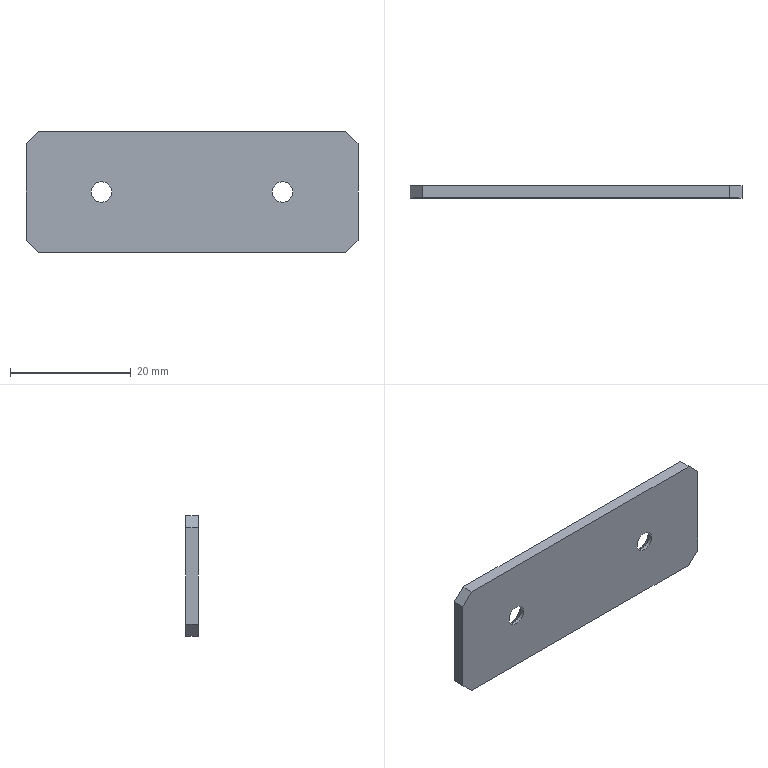Part | STEP file | Part1.SLDPRTrtt_Default | 1 solid | 18 faces | box 55 x 2 x 20 mm | volume 2119 mm3 | plane 10 | cone 4 | cylinder 4 | commonest cylinder face diameters 3.4 x4
STEP:
#1=CARTESIAN_POINT('',(0.,0.,0.));
#2=DIRECTION('',(0.,0.,1.));
#3=DIRECTION('',(1.,0.,0.));
#4=AXIS2_PLACEMENT_3D('',#1,#2,#3);
#5=CARTESIAN_POINT('',(-15.,0.55,1.7));
#6=VERTEX_POINT('',#5);
#7=CARTESIAN_POINT('',(-15.,2.,3.15));
#8=VERTEX_POINT('',#7);
#9=CARTESIAN_POINT('',(-15.,2.,3.15));
#10=DIRECTION('',(0.,0.7071,0.7071));
#11=VECTOR('',#10,1.);
#12=LINE('',#9,#11);
#13=CARTESIAN_POINT('',(-15.,2.,0.));
#14=DIRECTION('',(0.,1.,0.));
#15=DIRECTION('',(0.,0.,1.));
#16=AXIS2_PLACEMENT_3D('',#13,#14,#15);
#17=CONICAL_SURFACE('',#16,3.15,0.7854);
#18=CARTESIAN_POINT('',(6.283,0.));
#19=DIRECTION('',(0.,1.));
#20=VECTOR('',#19,1.);
#21=LINE('',#18,#20);
#22=(GEOMETRIC_REPRESENTATION_CONTEXT(2)PARAMETRIC_REPRESENTATION_CONTEXT()REPRESENTATION_CONTEXT('',''));
#23=DEFINITIONAL_REPRESENTATION('',(#21),#22);
#24=PCURVE('',#17,#23);
#25=CARTESIAN_POINT('',(-15.,2.,0.));
#26=DIRECTION('',(0.,1.,0.));
#27=DIRECTION('',(0.,0.,1.));
#28=AXIS2_PLACEMENT_3D('',#25,#26,#27);
#29=CONICAL_SURFACE('',#28,3.15,0.7854);
#30=CARTESIAN_POINT('',(0.,0.));
#31=DIRECTION('',(0.,1.));
#32=VECTOR('',#31,1.);
#33=LINE('',#30,#32);
#34=(GEOMETRIC_REPRESENTATION_CONTEXT(2)PARAMETRIC_REPRESENTATION_CONTEXT()REPRESENTATION_CONTEXT('',''));
#35=DEFINITIONAL_REPRESENTATION('',(#33),#34);
#36=PCURVE('',#29,#35);
#37=SURFACE_CURVE('',#12,(#24,#36),.PCURVE_S1.);
#38=EDGE_CURVE('',#6,#8,#37,.T.);
#39=ORIENTED_EDGE('',*,*,#38,.T.);
#40=CARTESIAN_POINT('',(-15.,2.,-3.15));
#41=VERTEX_POINT('',#40);
#42=CARTESIAN_POINT('',(-15.,2.,0.));
#43=DIRECTION('',(0.,1.,0.));
#44=DIRECTION('',(0.,0.,1.));
#45=AXIS2_PLACEMENT_3D('',#42,#43,#44);
#46=CIRCLE('',#45,3.15);
#47=CARTESIAN_POINT('',(0.,0.));
#48=DIRECTION('',(1.,0.));
#49=VECTOR('',#48,1.);
#50=LINE('',#47,#49);
#51=(GEOMETRIC_REPRESENTATION_CONTEXT(2)PARAMETRIC_REPRESENTATION_CONTEXT()REPRESENTATION_CONTEXT('',''));
#52=DEFINITIONAL_REPRESENTATION('',(#50),#51);
#53=PCURVE('',#17,#52);
#54=CARTESIAN_POINT('',(0.,2.,0.));
#55=DIRECTION('',(0.,1.,0.));
#56=DIRECTION('',(0.,0.,1.));
#57=AXIS2_PLACEMENT_3D('',#54,#55,#56);
#58=PLANE('',#57);
#59=CARTESIAN_POINT('',(0.,-15.));
#60=DIRECTION('',(1.,0.));
#61=AXIS2_PLACEMENT_2D('',#59,#60);
#62=CIRCLE('',#61,3.15);
#63=(GEOMETRIC_REPRESENTATION_CONTEXT(2)PARAMETRIC_REPRESENTATION_CONTEXT()REPRESENTATION_CONTEXT('',''));
#64=DEFINITIONAL_REPRESENTATION('',(#62),#63);
#65=PCURVE('',#58,#64);
#66=SURFACE_CURVE('',#46,(#53,#65),.PCURVE_S1.);
#67=EDGE_CURVE('',#41,#8,#66,.T.);
#68=ORIENTED_EDGE('',*,*,#67,.F.);
#69=CARTESIAN_POINT('',(-15.,0.55,-1.7));
#70=VERTEX_POINT('',#69);
#71=CARTESIAN_POINT('',(-15.,2.,-3.15));
#72=DIRECTION('',(0.,0.7071,-0.7071));
#73=VECTOR('',#72,1.);
#74=LINE('',#71,#73);
#75=CARTESIAN_POINT('',(3.142,0.));
#76=DIRECTION('',(0.,1.));
#77=VECTOR('',#76,1.);
#78=LINE('',#75,#77);
#79=(GEOMETRIC_REPRESENTATION_CONTEXT(2)PARAMETRIC_REPRESENTATION_CONTEXT()REPRESENTATION_CONTEXT('',''));
#80=DEFINITIONAL_REPRESENTATION('',(#78),#79);
#81=PCURVE('',#17,#80);
#82=CARTESIAN_POINT('',(3.142,0.));
#83=DIRECTION('',(0.,1.));
#84=VECTOR('',#83,1.);
#85=LINE('',#82,#84);
#86=(GEOMETRIC_REPRESENTATION_CONTEXT(2)PARAMETRIC_REPRESENTATION_CONTEXT()REPRESENTATION_CONTEXT('',''));
#87=DEFINITIONAL_REPRESENTATION('',(#85),#86);
#88=PCURVE('',#29,#87);
#89=SURFACE_CURVE('',#74,(#81,#88),.PCURVE_S1.);
#90=EDGE_CURVE('',#70,#41,#89,.T.);
#91=ORIENTED_EDGE('',*,*,#90,.F.);
#92=CARTESIAN_POINT('',(-15.,0.55,0.));
#93=DIRECTION('',(0.,1.,0.));
#94=DIRECTION('',(0.,0.,1.));
#95=AXIS2_PLACEMENT_3D('',#92,#93,#94);
#96=CIRCLE('',#95,1.7);
#97=CARTESIAN_POINT('',(0.,-1.45));
#98=DIRECTION('',(1.,0.));
#99=VECTOR('',#98,1.);
#100=LINE('',#97,#99);
#101=(GEOMETRIC_REPRESENTATION_CONTEXT(2)PARAMETRIC_REPRESENTATION_CONTEXT()REPRESENTATION_CONTEXT('',''));
#102=DEFINITIONAL_REPRESENTATION('',(#100),#101);
#103=PCURVE('',#17,#102);
#104=CARTESIAN_POINT('',(-15.,2.,0.));
#105=DIRECTION('',(0.,1.,0.));
#106=DIRECTION('',(0.,0.,1.));
#107=AXIS2_PLACEMENT_3D('',#104,#105,#106);
#108=CYLINDRICAL_SURFACE('',#107,1.7);
#109=CARTESIAN_POINT('',(0.,-1.45));
#110=DIRECTION('',(1.,0.));
#111=VECTOR('',#110,1.);
#112=LINE('',#109,#111);
#113=(GEOMETRIC_REPRESENTATION_CONTEXT(2)PARAMETRIC_REPRESENTATION_CONTEXT()REPRESENTATION_CONTEXT('',''));
#114=DEFINITIONAL_REPRESENTATION('',(#112),#113);
#115=PCURVE('',#108,#114);
#116=SURFACE_CURVE('',#96,(#103,#115),.PCURVE_S1.);
#117=EDGE_CURVE('',#70,#6,#116,.T.);
#118=ORIENTED_EDGE('',*,*,#117,.T.);
#119=EDGE_LOOP('',(#39,#68,#91,#118));
#120=FACE_BOUND('',#119,.F.);
#121=ADVANCED_FACE('',(#120),#17,.F.);
#122=CARTESIAN_POINT('',(-15.,0.,1.7));
#123=VERTEX_POINT('',#122);
#124=CARTESIAN_POINT('',(-15.,2.,1.7));
#125=DIRECTION('',(0.,1.,0.));
#126=VECTOR('',#125,1.);
#127=LINE('',#124,#126);
#128=CARTESIAN_POINT('',(6.283,0.));
#129=DIRECTION('',(0.,1.));
#130=VECTOR('',#129,1.);
#131=LINE('',#128,#130);
#132=(GEOMETRIC_REPRESENTATION_CONTEXT(2)PARAMETRIC_REPRESENTATION_CONTEXT()REPRESENTATION_CONTEXT('',''));
#133=DEFINITIONAL_REPRESENTATION('',(#131),#132);
#134=PCURVE('',#108,#133);
#135=CARTESIAN_POINT('',(-15.,2.,0.));
#136=DIRECTION('',(0.,1.,0.));
#137=DIRECTION('',(0.,0.,1.));
#138=AXIS2_PLACEMENT_3D('',#135,#136,#137);
#139=CYLINDRICAL_SURFACE('',#138,1.7);
#140=CARTESIAN_POINT('',(0.,0.));
#141=DIRECTION('',(0.,1.));
#142=VECTOR('',#141,1.);
#143=LINE('',#140,#142);
#144=(GEOMETRIC_REPRESENTATION_CONTEXT(2)PARAMETRIC_REPRESENTATION_CONTEXT()REPRESENTATION_CONTEXT('',''));
#145=DEFINITIONAL_REPRESENTATION('',(#143),#144);
#146=PCURVE('',#139,#145);
#147=SURFACE_CURVE('',#127,(#134,#146),.PCURVE_S1.);
#148=EDGE_CURVE('',#123,#6,#147,.T.);
#149=ORIENTED_EDGE('',*,*,#148,.T.);
#150=ORIENTED_EDGE('',*,*,#117,.F.);
#151=CARTESIAN_POINT('',(-15.,0.,-1.7));
#152=VERTEX_POINT('',#151);
#153=CARTESIAN_POINT('',(-15.,2.,-1.7));
#154=DIRECTION('',(0.,1.,0.));
#155=VECTOR('',#154,1.);
#156=LINE('',#153,#155);
#157=CARTESIAN_POINT('',(3.142,0.));
#158=DIRECTION('',(0.,1.));
#159=VECTOR('',#158,1.);
#160=LINE('',#157,#159);
#161=(GEOMETRIC_REPRESENTATION_CONTEXT(2)PARAMETRIC_REPRESENTATION_CONTEXT()REPRESENTATION_CONTEXT('',''));
#162=DEFINITIONAL_REPRESENTATION('',(#160),#161);
#163=PCURVE('',#108,#162);
#164=CARTESIAN_POINT('',(3.142,0.));
#165=DIRECTION('',(0.,1.));
#166=VECTOR('',#165,1.);
#167=LINE('',#164,#166);
#168=(GEOMETRIC_REPRESENTATION_CONTEXT(2)PARAMETRIC_REPRESENTATION_CONTEXT()REPRESENTATION_CONTEXT('',''));
#169=DEFINITIONAL_REPRESENTATION('',(#167),#168);
#170=PCURVE('',#139,#169);
#171=SURFACE_CURVE('',#156,(#163,#170),.PCURVE_S1.);
#172=EDGE_CURVE('',#152,#70,#171,.T.);
#173=ORIENTED_EDGE('',*,*,#172,.F.);
#174=CARTESIAN_POINT('',(-15.,0.,0.));
#175=DIRECTION('',(0.,1.,0.));
#176=DIRECTION('',(0.,0.,1.));
#177=AXIS2_PLACEMENT_3D('',#174,#175,#176);
#178=CIRCLE('',#177,1.7);
#179=CARTESIAN_POINT('',(0.,-2.));
#180=DIRECTION('',(1.,0.));
#181=VECTOR('',#180,1.);
#182=LINE('',#179,#181);
#183=(GEOMETRIC_REPRESENTATION_CONTEXT(2)PARAMETRIC_REPRESENTATION_CONTEXT()REPRESENTATION_CONTEXT('',''));
#184=DEFINITIONAL_REPRESENTATION('',(#182),#183);
#185=PCURVE('',#108,#184);
#186=CARTESIAN_POINT('',(0.,0.,0.));
#187=DIRECTION('',(0.,1.,0.));
#188=DIRECTION('',(0.,0.,1.));
#189=AXIS2_PLACEMENT_3D('',#186,#187,#188);
#190=PLANE('',#189);
#191=CARTESIAN_POINT('',(0.,-15.));
#192=DIRECTION('',(1.,0.));
#193=AXIS2_PLACEMENT_2D('',#191,#192);
#194=CIRCLE('',#193,1.7);
#195=(GEOMETRIC_REPRESENTATION_CONTEXT(2)PARAMETRIC_REPRESENTATION_CONTEXT()REPRESENTATION_CONTEXT('',''));
#196=DEFINITIONAL_REPRESENTATION('',(#194),#195);
#197=PCURVE('',#190,#196);
#198=SURFACE_CURVE('',#178,(#185,#197),.PCURVE_S1.);
#199=EDGE_CURVE('',#152,#123,#198,.T.);
#200=ORIENTED_EDGE('',*,*,#199,.T.);
#201=EDGE_LOOP('',(#149,#150,#173,#200));
#202=FACE_BOUND('',#201,.F.);
#203=ADVANCED_FACE('',(#202),#108,.F.);
#204=CARTESIAN_POINT('',(15.,0.55,1.7));
#205=VERTEX_POINT('',#204);
#206=CARTESIAN_POINT('',(15.,2.,3.15));
#207=VERTEX_POINT('',#206);
#208=CARTESIAN_POINT('',(15.,2.,3.15));
#209=DIRECTION('',(0.,0.7071,0.7071));
#210=VECTOR('',#209,1.);
#211=LINE('',#208,#210);
#212=CARTESIAN_POINT('',(15.,2.,0.));
#213=DIRECTION('',(0.,1.,0.));
#214=DIRECTION('',(0.,0.,1.));
#215=AXIS2_PLACEMENT_3D('',#212,#213,#214);
#216=CONICAL_SURFACE('',#215,3.15,0.7854);
#217=CARTESIAN_POINT('',(6.283,0.));
#218=DIRECTION('',(0.,1.));
#219=VECTOR('',#218,1.);
#220=LINE('',#217,#219);
#221=(GEOMETRIC_REPRESENTATION_CONTEXT(2)PARAMETRIC_REPRESENTATION_CONTEXT()REPRESENTATION_CONTEXT('',''));
#222=DEFINITIONAL_REPRESENTATION('',(#220),#221);
#223=PCURVE('',#216,#222);
#224=CARTESIAN_POINT('',(15.,2.,0.));
#225=DIRECTION('',(0.,1.,0.));
#226=DIRECTION('',(0.,0.,1.));
#227=AXIS2_PLACEMENT_3D('',#224,#225,#226);
#228=CONICAL_SURFACE('',#227,3.15,0.7854);
#229=CARTESIAN_POINT('',(0.,0.));
#230=DIRECTION('',(0.,1.));
#231=VECTOR('',#230,1.);
#232=LINE('',#229,#231);
#233=(GEOMETRIC_REPRESENTATION_CONTEXT(2)PARAMETRIC_REPRESENTATION_CONTEXT()REPRESENTATION_CONTEXT('',''));
#234=DEFINITIONAL_REPRESENTATION('',(#232),#233);
#235=PCURVE('',#228,#234);
#236=SURFACE_CURVE('',#211,(#223,#235),.PCURVE_S1.);
#237=EDGE_CURVE('',#205,#207,#236,.T.);
#238=ORIENTED_EDGE('',*,*,#237,.T.);
#239=CARTESIAN_POINT('',(15.,2.,-3.15));
#240=VERTEX_POINT('',#239);
#241=CARTESIAN_POINT('',(15.,2.,0.));
#242=DIRECTION('',(0.,1.,0.));
#243=DIRECTION('',(0.,0.,1.));
#244=AXIS2_PLACEMENT_3D('',#241,#242,#243);
#245=CIRCLE('',#244,3.15);
#246=CARTESIAN_POINT('',(0.,0.));
#247=DIRECTION('',(1.,0.));
#248=VECTOR('',#247,1.);
#249=LINE('',#246,#248);
#250=(GEOMETRIC_REPRESENTATION_CONTEXT(2)PARAMETRIC_REPRESENTATION_CONTEXT()REPRESENTATION_CONTEXT('',''));
#251=DEFINITIONAL_REPRESENTATION('',(#249),#250);
#252=PCURVE('',#216,#251);
#253=CARTESIAN_POINT('',(0.,15.));
#254=DIRECTION('',(1.,0.));
#255=AXIS2_PLACEMENT_2D('',#253,#254);
#256=CIRCLE('',#255,3.15);
#257=(GEOMETRIC_REPRESENTATION_CONTEXT(2)PARAMETRIC_REPRESENTATION_CONTEXT()REPRESENTATION_CONTEXT('',''));
#258=DEFINITIONAL_REPRESENTATION('',(#256),#257);
#259=PCURVE('',#58,#258);
#260=SURFACE_CURVE('',#245,(#252,#259),.PCURVE_S1.);
#261=EDGE_CURVE('',#240,#207,#260,.T.);
#262=ORIENTED_EDGE('',*,*,#261,.F.);
#263=CARTESIAN_POINT('',(15.,0.55,-1.7));
#264=VERTEX_POINT('',#263);
#265=CARTESIAN_POINT('',(15.,2.,-3.15));
#266=DIRECTION('',(0.,0.7071,-0.7071));
#267=VECTOR('',#266,1.);
#268=LINE('',#265,#267);
#269=CARTESIAN_POINT('',(3.142,0.));
#270=DIRECTION('',(0.,1.));
#271=VECTOR('',#270,1.);
#272=LINE('',#269,#271);
#273=(GEOMETRIC_REPRESENTATION_CONTEXT(2)PARAMETRIC_REPRESENTATION_CONTEXT()REPRESENTATION_CONTEXT('',''));
#274=DEFINITIONAL_REPRESENTATION('',(#272),#273);
#275=PCURVE('',#216,#274);
#276=CARTESIAN_POINT('',(3.142,0.));
#277=DIRECTION('',(0.,1.));
#278=VECTOR('',#277,1.);
#279=LINE('',#276,#278);
#280=(GEOMETRIC_REPRESENTATION_CONTEXT(2)PARAMETRIC_REPRESENTATION_CONTEXT()REPRESENTATION_CONTEXT('',''));
#281=DEFINITIONAL_REPRESENTATION('',(#279),#280);
#282=PCURVE('',#228,#281);
#283=SURFACE_CURVE('',#268,(#275,#282),.PCURVE_S1.);
#284=EDGE_CURVE('',#264,#240,#283,.T.);
#285=ORIENTED_EDGE('',*,*,#284,.F.);
#286=CARTESIAN_POINT('',(15.,0.55,0.));
#287=DIRECTION('',(0.,1.,0.));
#288=DIRECTION('',(0.,0.,1.));
#289=AXIS2_PLACEMENT_3D('',#286,#287,#288);
#290=CIRCLE('',#289,1.7);
#291=CARTESIAN_POINT('',(0.,-1.45));
#292=DIRECTION('',(1.,0.));
#293=VECTOR('',#292,1.);
#294=LINE('',#291,#293);
#295=(GEOMETRIC_REPRESENTATION_CONTEXT(2)PARAMETRIC_REPRESENTATION_CONTEXT()REPRESENTATION_CONTEXT('',''));
#296=DEFINITIONAL_REPRESENTATION('',(#294),#295);
#297=PCURVE('',#216,#296);
#298=CARTESIAN_POINT('',(15.,2.,0.));
#299=DIRECTION('',(0.,1.,0.));
#300=DIRECTION('',(0.,0.,1.));
#301=AXIS2_PLACEMENT_3D('',#298,#299,#300);
#302=CYLINDRICAL_SURFACE('',#301,1.7);
#303=CARTESIAN_POINT('',(0.,-1.45));
#304=DIRECTION('',(1.,0.));
#305=VECTOR('',#304,1.);
#306=LINE('',#303,#305);
#307=(GEOMETRIC_REPRESENTATION_CONTEXT(2)PARAMETRIC_REPRESENTATION_CONTEXT()REPRESENTATION_CONTEXT('',''));
#308=DEFINITIONAL_REPRESENTATION('',(#306),#307);
#309=PCURVE('',#302,#308);
#310=SURFACE_CURVE('',#290,(#297,#309),.PCURVE_S1.);
#311=EDGE_CURVE('',#264,#205,#310,.T.);
#312=ORIENTED_EDGE('',*,*,#311,.T.);
#313=EDGE_LOOP('',(#238,#262,#285,#312));
#314=FACE_BOUND('',#313,.F.);
#315=ADVANCED_FACE('',(#314),#216,.F.);
#316=CARTESIAN_POINT('',(15.,0.,1.7));
#317=VERTEX_POINT('',#316);
#318=CARTESIAN_POINT('',(15.,2.,1.7));
#319=DIRECTION('',(0.,1.,0.));
#320=VECTOR('',#319,1.);
#321=LINE('',#318,#320);
#322=CARTESIAN_POINT('',(6.283,0.));
#323=DIRECTION('',(0.,1.));
#324=VECTOR('',#323,1.);
#325=LINE('',#322,#324);
#326=(GEOMETRIC_REPRESENTATION_CONTEXT(2)PARAMETRIC_REPRESENTATION_CONTEXT()REPRESENTATION_CONTEXT('',''));
#327=DEFINITIONAL_REPRESENTATION('',(#325),#326);
#328=PCURVE('',#302,#327);
#329=CARTESIAN_POINT('',(15.,2.,0.));
#330=DIRECTION('',(0.,1.,0.));
#331=DIRECTION('',(0.,0.,1.));
#332=AXIS2_PLACEMENT_3D('',#329,#330,#331);
#333=CYLINDRICAL_SURFACE('',#332,1.7);
#334=CARTESIAN_POINT('',(0.,0.));
#335=DIRECTION('',(0.,1.));
#336=VECTOR('',#335,1.);
#337=LINE('',#334,#336);
#338=(GEOMETRIC_REPRESENTATION_CONTEXT(2)PARAMETRIC_REPRESENTATION_CONTEXT()REPRESENTATION_CONTEXT('',''));
#339=DEFINITIONAL_REPRESENTATION('',(#337),#338);
#340=PCURVE('',#333,#339);
#341=SURFACE_CURVE('',#321,(#328,#340),.PCURVE_S1.);
#342=EDGE_CURVE('',#317,#205,#341,.T.);
#343=ORIENTED_EDGE('',*,*,#342,.T.);
#344=ORIENTED_EDGE('',*,*,#311,.F.);
#345=CARTESIAN_POINT('',(15.,0.,-1.7));
#346=VERTEX_POINT('',#345);
#347=CARTESIAN_POINT('',(15.,2.,-1.7));
#348=DIRECTION('',(0.,1.,0.));
#349=VECTOR('',#348,1.);
#350=LINE('',#347,#349);
#351=CARTESIAN_POINT('',(3.142,0.));
#352=DIRECTION('',(0.,1.));
#353=VECTOR('',#352,1.);
#354=LINE('',#351,#353);
#355=(GEOMETRIC_REPRESENTATION_CONTEXT(2)PARAMETRIC_REPRESENTATION_CONTEXT()REPRESENTATION_CONTEXT('',''));
#356=DEFINITIONAL_REPRESENTATION('',(#354),#355);
#357=PCURVE('',#302,#356);
#358=CARTESIAN_POINT('',(3.142,0.));
#359=DIRECTION('',(0.,1.));
#360=VECTOR('',#359,1.);
#361=LINE('',#358,#360);
#362=(GEOMETRIC_REPRESENTATION_CONTEXT(2)PARAMETRIC_REPRESENTATION_CONTEXT()REPRESENTATION_CONTEXT('',''));
#363=DEFINITIONAL_REPRESENTATION('',(#361),#362);
#364=PCURVE('',#333,#363);
#365=SURFACE_CURVE('',#350,(#357,#364),.PCURVE_S1.);
#366=EDGE_CURVE('',#346,#264,#365,.T.);
#367=ORIENTED_EDGE('',*,*,#366,.F.);
#368=CARTESIAN_POINT('',(15.,0.,0.));
#369=DIRECTION('',(0.,1.,0.));
#370=DIRECTION('',(0.,0.,1.));
#371=AXIS2_PLACEMENT_3D('',#368,#369,#370);
#372=CIRCLE('',#371,1.7);
#373=CARTESIAN_POINT('',(0.,-2.));
#374=DIRECTION('',(1.,0.));
#375=VECTOR('',#374,1.);
#376=LINE('',#373,#375);
#377=(GEOMETRIC_REPRESENTATION_CONTEXT(2)PARAMETRIC_REPRESENTATION_CONTEXT()REPRESENTATION_CONTEXT('',''));
#378=DEFINITIONAL_REPRESENTATION('',(#376),#377);
#379=PCURVE('',#302,#378);
#380=CARTESIAN_POINT('',(0.,15.));
#381=DIRECTION('',(1.,0.));
#382=AXIS2_PLACEMENT_2D('',#380,#381);
#383=CIRCLE('',#382,1.7);
#384=(GEOMETRIC_REPRESENTATION_CONTEXT(2)PARAMETRIC_REPRESENTATION_CONTEXT()REPRESENTATION_CONTEXT('',''));
#385=DEFINITIONAL_REPRESENTATION('',(#383),#384);
#386=PCURVE('',#190,#385);
#387=SURFACE_CURVE('',#372,(#379,#386),.PCURVE_S1.);
#388=EDGE_CURVE('',#346,#317,#387,.T.);
#389=ORIENTED_EDGE('',*,*,#388,.T.);
#390=EDGE_LOOP('',(#343,#344,#367,#389));
#391=FACE_BOUND('',#390,.F.);
#392=ADVANCED_FACE('',(#391),#302,.F.);
#393=CARTESIAN_POINT('',(-27.5,0.,-8.));
#394=VERTEX_POINT('',#393);
#395=CARTESIAN_POINT('',(-27.5,0.,8.));
#396=VERTEX_POINT('',#395);
#397=CARTESIAN_POINT('',(-27.5,0.,10.));
#398=DIRECTION('',(0.,0.,1.));
#399=VECTOR('',#398,1.);
#400=LINE('',#397,#399);
#401=CARTESIAN_POINT('',(-27.5,2.,10.));
#402=DIRECTION('',(1.,0.,0.));
#403=DIRECTION('',(0.,0.,-1.));
#404=AXIS2_PLACEMENT_3D('',#401,#402,#403);
#405=PLANE('',#404);
#406=CARTESIAN_POINT('',(0.,-2.));
#407=DIRECTION('',(-1.,0.));
#408=VECTOR('',#407,1.);
#409=LINE('',#406,#408);
#410=(GEOMETRIC_REPRESENTATION_CONTEXT(2)PARAMETRIC_REPRESENTATION_CONTEXT()REPRESENTATION_CONTEXT('',''));
#411=DEFINITIONAL_REPRESENTATION('',(#409),#410);
#412=PCURVE('',#405,#411);
#413=CARTESIAN_POINT('',(10.,-27.5));
#414=DIRECTION('',(1.,0.));
#415=VECTOR('',#414,1.);
#416=LINE('',#413,#415);
#417=(GEOMETRIC_REPRESENTATION_CONTEXT(2)PARAMETRIC_REPRESENTATION_CONTEXT()REPRESENTATION_CONTEXT('',''));
#418=DEFINITIONAL_REPRESENTATION('',(#416),#417);
#419=PCURVE('',#190,#418);
#420=SURFACE_CURVE('',#400,(#412,#419),.PCURVE_S1.);
#421=EDGE_CURVE('',#394,#396,#420,.T.);
#422=ORIENTED_EDGE('',*,*,#421,.T.);
#423=CARTESIAN_POINT('',(-27.5,2.,8.));
#424=VERTEX_POINT('',#423);
#425=CARTESIAN_POINT('',(-27.5,2.,8.));
#426=DIRECTION('',(0.,1.,0.));
#427=VECTOR('',#426,1.);
#428=LINE('',#425,#427);
#429=CARTESIAN_POINT('',(2.,0.));
#430=DIRECTION('',(0.,1.));
#431=VECTOR('',#430,1.);
#432=LINE('',#429,#431);
#433=(GEOMETRIC_REPRESENTATION_CONTEXT(2)PARAMETRIC_REPRESENTATION_CONTEXT()REPRESENTATION_CONTEXT('',''));
#434=DEFINITIONAL_REPRESENTATION('',(#432),#433);
#435=PCURVE('',#405,#434);
#436=CARTESIAN_POINT('',(-25.5,2.,10.));
#437=DIRECTION('',(0.7071,0.,-0.7071));
#438=DIRECTION('',(0.,-1.,0.));
#439=AXIS2_PLACEMENT_3D('',#436,#437,#438);
#440=PLANE('',#439);
#441=CARTESIAN_POINT('',(0.,2.828));
#442=DIRECTION('',(-1.,0.));
#443=VECTOR('',#442,1.);
#444=LINE('',#441,#443);
#445=(GEOMETRIC_REPRESENTATION_CONTEXT(2)PARAMETRIC_REPRESENTATION_CONTEXT()REPRESENTATION_CONTEXT('',''));
#446=DEFINITIONAL_REPRESENTATION('',(#444),#445);
#447=PCURVE('',#440,#446);
#448=SURFACE_CURVE('',#428,(#435,#447),.PCURVE_S1.);
#449=EDGE_CURVE('',#396,#424,#448,.T.);
#450=ORIENTED_EDGE('',*,*,#449,.T.);
#451=CARTESIAN_POINT('',(-27.5,2.,-8.));
#452=VERTEX_POINT('',#451);
#453=CARTESIAN_POINT('',(-27.5,2.,10.));
#454=DIRECTION('',(0.,0.,1.));
#455=VECTOR('',#454,1.);
#456=LINE('',#453,#455);
#457=CARTESIAN_POINT('',(0.,0.));
#458=DIRECTION('',(-1.,0.));
#459=VECTOR('',#458,1.);
#460=LINE('',#457,#459);
#461=(GEOMETRIC_REPRESENTATION_CONTEXT(2)PARAMETRIC_REPRESENTATION_CONTEXT()REPRESENTATION_CONTEXT('',''));
#462=DEFINITIONAL_REPRESENTATION('',(#460),#461);
#463=PCURVE('',#405,#462);
#464=CARTESIAN_POINT('',(10.,-27.5));
#465=DIRECTION('',(1.,0.));
#466=VECTOR('',#465,1.);
#467=LINE('',#464,#466);
#468=(GEOMETRIC_REPRESENTATION_CONTEXT(2)PARAMETRIC_REPRESENTATION_CONTEXT()REPRESENTATION_CONTEXT('',''));
#469=DEFINITIONAL_REPRESENTATION('',(#467),#468);
#470=PCURVE('',#58,#469);
#471=SURFACE_CURVE('',#456,(#463,#470),.PCURVE_S1.);
#472=EDGE_CURVE('',#452,#424,#471,.T.);
#473=ORIENTED_EDGE('',*,*,#472,.F.);
#474=CARTESIAN_POINT('',(-27.5,2.,-8.));
#475=DIRECTION('',(0.,-1.,0.));
#476=VECTOR('',#475,1.);
#477=LINE('',#474,#476);
#478=CARTESIAN_POINT('',(18.,0.));
#479=DIRECTION('',(0.,-1.));
#480=VECTOR('',#479,1.);
#481=LINE('',#478,#480);
#482=(GEOMETRIC_REPRESENTATION_CONTEXT(2)PARAMETRIC_REPRESENTATION_CONTEXT()REPRESENTATION_CONTEXT('',''));
#483=DEFINITIONAL_REPRESENTATION('',(#481),#482);
#484=PCURVE('',#405,#483);
#485=CARTESIAN_POINT('',(-27.5,2.,-8.));
#486=DIRECTION('',(0.7071,0.,0.7071));
#487=DIRECTION('',(0.,-1.,0.));
#488=AXIS2_PLACEMENT_3D('',#485,#486,#487);
#489=PLANE('',#488);
#490=CARTESIAN_POINT('',(0.,0.));
#491=DIRECTION('',(1.,0.));
#492=VECTOR('',#491,1.);
#493=LINE('',#490,#492);
#494=(GEOMETRIC_REPRESENTATION_CONTEXT(2)PARAMETRIC_REPRESENTATION_CONTEXT()REPRESENTATION_CONTEXT('',''));
#495=DEFINITIONAL_REPRESENTATION('',(#493),#494);
#496=PCURVE('',#489,#495);
#497=SURFACE_CURVE('',#477,(#484,#496),.PCURVE_S1.);
#498=EDGE_CURVE('',#452,#394,#497,.T.);
#499=ORIENTED_EDGE('',*,*,#498,.T.);
#500=EDGE_LOOP('',(#422,#450,#473,#499));
#501=FACE_BOUND('',#500,.T.);
#502=ADVANCED_FACE('',(#501),#405,.F.);
#503=CARTESIAN_POINT('',(-25.5,2.,10.));
#504=VERTEX_POINT('',#503);
#505=CARTESIAN_POINT('',(25.5,2.,10.));
#506=VERTEX_POINT('',#505);
#507=CARTESIAN_POINT('',(27.5,2.,10.));
#508=DIRECTION('',(1.,0.,0.));
#509=VECTOR('',#508,1.);
#510=LINE('',#507,#509);
#511=CARTESIAN_POINT('',(27.5,2.,10.));
#512=DIRECTION('',(0.,0.,-1.));
#513=DIRECTION('',(-1.,0.,0.));
#514=AXIS2_PLACEMENT_3D('',#511,#512,#513);
#515=PLANE('',#514);
#516=CARTESIAN_POINT('',(0.,0.));
#517=DIRECTION('',(-1.,0.));
#518=VECTOR('',#517,1.);
#519=LINE('',#516,#518);
#520=(GEOMETRIC_REPRESENTATION_CONTEXT(2)PARAMETRIC_REPRESENTATION_CONTEXT()REPRESENTATION_CONTEXT('',''));
#521=DEFINITIONAL_REPRESENTATION('',(#519),#520);
#522=PCURVE('',#515,#521);
#523=CARTESIAN_POINT('',(10.,27.5));
#524=DIRECTION('',(0.,1.));
#525=VECTOR('',#524,1.);
#526=LINE('',#523,#525);
#527=(GEOMETRIC_REPRESENTATION_CONTEXT(2)PARAMETRIC_REPRESENTATION_CONTEXT()REPRESENTATION_CONTEXT('',''));
#528=DEFINITIONAL_REPRESENTATION('',(#526),#527);
#529=PCURVE('',#58,#528);
#530=SURFACE_CURVE('',#510,(#522,#529),.PCURVE_S1.);
#531=EDGE_CURVE('',#504,#506,#530,.T.);
#532=ORIENTED_EDGE('',*,*,#531,.F.);
#533=CARTESIAN_POINT('',(-25.5,0.,10.));
#534=VERTEX_POINT('',#533);
#535=CARTESIAN_POINT('',(-25.5,2.,10.));
#536=DIRECTION('',(0.,-1.,0.));
#537=VECTOR('',#536,1.);
#538=LINE('',#535,#537);
#539=CARTESIAN_POINT('',(53.,0.));
#540=DIRECTION('',(0.,-1.));
#541=VECTOR('',#540,1.);
#542=LINE('',#539,#541);
#543=(GEOMETRIC_REPRESENTATION_CONTEXT(2)PARAMETRIC_REPRESENTATION_CONTEXT()REPRESENTATION_CONTEXT('',''));
#544=DEFINITIONAL_REPRESENTATION('',(#542),#543);
#545=PCURVE('',#515,#544);
#546=CARTESIAN_POINT('',(0.,0.));
#547=DIRECTION('',(1.,0.));
#548=VECTOR('',#547,1.);
#549=LINE('',#546,#548);
#550=(GEOMETRIC_REPRESENTATION_CONTEXT(2)PARAMETRIC_REPRESENTATION_CONTEXT()REPRESENTATION_CONTEXT('',''));
#551=DEFINITIONAL_REPRESENTATION('',(#549),#550);
#552=PCURVE('',#440,#551);
#553=SURFACE_CURVE('',#538,(#545,#552),.PCURVE_S1.);
#554=EDGE_CURVE('',#504,#534,#553,.T.);
#555=ORIENTED_EDGE('',*,*,#554,.T.);
#556=CARTESIAN_POINT('',(25.5,0.,10.));
#557=VERTEX_POINT('',#556);
#558=CARTESIAN_POINT('',(27.5,0.,10.));
#559=DIRECTION('',(1.,0.,0.));
#560=VECTOR('',#559,1.);
#561=LINE('',#558,#560);
#562=CARTESIAN_POINT('',(0.,-2.));
#563=DIRECTION('',(-1.,0.));
#564=VECTOR('',#563,1.);
#565=LINE('',#562,#564);
#566=(GEOMETRIC_REPRESENTATION_CONTEXT(2)PARAMETRIC_REPRESENTATION_CONTEXT()REPRESENTATION_CONTEXT('',''));
#567=DEFINITIONAL_REPRESENTATION('',(#565),#566);
#568=PCURVE('',#515,#567);
#569=CARTESIAN_POINT('',(10.,27.5));
#570=DIRECTION('',(0.,1.));
#571=VECTOR('',#570,1.);
#572=LINE('',#569,#571);
#573=(GEOMETRIC_REPRESENTATION_CONTEXT(2)PARAMETRIC_REPRESENTATION_CONTEXT()REPRESENTATION_CONTEXT('',''));
#574=DEFINITIONAL_REPRESENTATION('',(#572),#573);
#575=PCURVE('',#190,#574);
#576=SURFACE_CURVE('',#561,(#568,#575),.PCURVE_S1.);
#577=EDGE_CURVE('',#534,#557,#576,.T.);
#578=ORIENTED_EDGE('',*,*,#577,.T.);
#579=CARTESIAN_POINT('',(25.5,2.,10.));
#580=DIRECTION('',(0.,1.,0.));
#581=VECTOR('',#580,1.);
#582=LINE('',#579,#581);
#583=CARTESIAN_POINT('',(2.,0.));
#584=DIRECTION('',(0.,1.));
#585=VECTOR('',#584,1.);
#586=LINE('',#583,#585);
#587=(GEOMETRIC_REPRESENTATION_CONTEXT(2)PARAMETRIC_REPRESENTATION_CONTEXT()REPRESENTATION_CONTEXT('',''));
#588=DEFINITIONAL_REPRESENTATION('',(#586),#587);
#589=PCURVE('',#515,#588);
#590=CARTESIAN_POINT('',(27.5,2.,8.));
#591=DIRECTION('',(-0.7071,0.,-0.7071));
#592=DIRECTION('',(0.,-1.,0.));
#593=AXIS2_PLACEMENT_3D('',#590,#591,#592);
#594=PLANE('',#593);
#595=CARTESIAN_POINT('',(0.,2.828));
#596=DIRECTION('',(-1.,0.));
#597=VECTOR('',#596,1.);
#598=LINE('',#595,#597);
#599=(GEOMETRIC_REPRESENTATION_CONTEXT(2)PARAMETRIC_REPRESENTATION_CONTEXT()REPRESENTATION_CONTEXT('',''));
#600=DEFINITIONAL_REPRESENTATION('',(#598),#599);
#601=PCURVE('',#594,#600);
#602=SURFACE_CURVE('',#582,(#589,#601),.PCURVE_S1.);
#603=EDGE_CURVE('',#557,#506,#602,.T.);
#604=ORIENTED_EDGE('',*,*,#603,.T.);
#605=EDGE_LOOP('',(#532,#555,#578,#604));
#606=FACE_BOUND('',#605,.T.);
#607=ADVANCED_FACE('',(#606),#515,.F.);
#608=CARTESIAN_POINT('',(27.5,2.,8.));
#609=VERTEX_POINT('',#608);
#610=CARTESIAN_POINT('',(27.5,2.,-8.));
#611=VERTEX_POINT('',#610);
#612=CARTESIAN_POINT('',(27.5,2.,10.));
#613=DIRECTION('',(0.,0.,-1.));
#614=VECTOR('',#613,1.);
#615=LINE('',#612,#614);
#616=CARTESIAN_POINT('',(27.5,2.,10.));
#617=DIRECTION('',(-1.,0.,0.));
#618=DIRECTION('',(0.,0.,1.));
#619=AXIS2_PLACEMENT_3D('',#616,#617,#618);
#620=PLANE('',#619);
#621=CARTESIAN_POINT('',(0.,0.));
#622=DIRECTION('',(-1.,0.));
#623=VECTOR('',#622,1.);
#624=LINE('',#621,#623);
#625=(GEOMETRIC_REPRESENTATION_CONTEXT(2)PARAMETRIC_REPRESENTATION_CONTEXT()REPRESENTATION_CONTEXT('',''));
#626=DEFINITIONAL_REPRESENTATION('',(#624),#625);
#627=PCURVE('',#620,#626);
#628=CARTESIAN_POINT('',(10.,27.5));
#629=DIRECTION('',(-1.,0.));
#630=VECTOR('',#629,1.);
#631=LINE('',#628,#630);
#632=(GEOMETRIC_REPRESENTATION_CONTEXT(2)PARAMETRIC_REPRESENTATION_CONTEXT()REPRESENTATION_CONTEXT('',''));
#633=DEFINITIONAL_REPRESENTATION('',(#631),#632);
#634=PCURVE('',#58,#633);
#635=SURFACE_CURVE('',#615,(#627,#634),.PCURVE_S1.);
#636=EDGE_CURVE('',#609,#611,#635,.T.);
#637=ORIENTED_EDGE('',*,*,#636,.F.);
#638=CARTESIAN_POINT('',(27.5,0.,8.));
#639=VERTEX_POINT('',#638);
#640=CARTESIAN_POINT('',(27.5,2.,8.));
#641=DIRECTION('',(0.,-1.,0.));
#642=VECTOR('',#641,1.);
#643=LINE('',#640,#642);
#644=CARTESIAN_POINT('',(-2.,0.));
#645=DIRECTION('',(0.,-1.));
#646=VECTOR('',#645,1.);
#647=LINE('',#644,#646);
#648=(GEOMETRIC_REPRESENTATION_CONTEXT(2)PARAMETRIC_REPRESENTATION_CONTEXT()REPRESENTATION_CONTEXT('',''));
#649=DEFINITIONAL_REPRESENTATION('',(#647),#648);
#650=PCURVE('',#620,#649);
#651=CARTESIAN_POINT('',(0.,0.));
#652=DIRECTION('',(1.,0.));
#653=VECTOR('',#652,1.);
#654=LINE('',#651,#653);
#655=(GEOMETRIC_REPRESENTATION_CONTEXT(2)PARAMETRIC_REPRESENTATION_CONTEXT()REPRESENTATION_CONTEXT('',''));
#656=DEFINITIONAL_REPRESENTATION('',(#654),#655);
#657=PCURVE('',#594,#656);
#658=SURFACE_CURVE('',#643,(#650,#657),.PCURVE_S1.);
#659=EDGE_CURVE('',#609,#639,#658,.T.);
#660=ORIENTED_EDGE('',*,*,#659,.T.);
#661=CARTESIAN_POINT('',(27.5,0.,-8.));
#662=VERTEX_POINT('',#661);
#663=CARTESIAN_POINT('',(27.5,0.,10.));
#664=DIRECTION('',(0.,0.,-1.));
#665=VECTOR('',#664,1.);
#666=LINE('',#663,#665);
#667=CARTESIAN_POINT('',(0.,-2.));
#668=DIRECTION('',(-1.,0.));
#669=VECTOR('',#668,1.);
#670=LINE('',#667,#669);
#671=(GEOMETRIC_REPRESENTATION_CONTEXT(2)PARAMETRIC_REPRESENTATION_CONTEXT()REPRESENTATION_CONTEXT('',''));
#672=DEFINITIONAL_REPRESENTATION('',(#670),#671);
#673=PCURVE('',#620,#672);
#674=CARTESIAN_POINT('',(10.,27.5));
#675=DIRECTION('',(-1.,0.));
#676=VECTOR('',#675,1.);
#677=LINE('',#674,#676);
#678=(GEOMETRIC_REPRESENTATION_CONTEXT(2)PARAMETRIC_REPRESENTATION_CONTEXT()REPRESENTATION_CONTEXT('',''));
#679=DEFINITIONAL_REPRESENTATION('',(#677),#678);
#680=PCURVE('',#190,#679);
#681=SURFACE_CURVE('',#666,(#673,#680),.PCURVE_S1.);
#682=EDGE_CURVE('',#639,#662,#681,.T.);
#683=ORIENTED_EDGE('',*,*,#682,.T.);
#684=CARTESIAN_POINT('',(27.5,2.,-8.));
#685=DIRECTION('',(0.,1.,0.));
#686=VECTOR('',#685,1.);
#687=LINE('',#684,#686);
#688=CARTESIAN_POINT('',(-18.,0.));
#689=DIRECTION('',(0.,1.));
#690=VECTOR('',#689,1.);
#691=LINE('',#688,#690);
#692=(GEOMETRIC_REPRESENTATION_CONTEXT(2)PARAMETRIC_REPRESENTATION_CONTEXT()REPRESENTATION_CONTEXT('',''));
#693=DEFINITIONAL_REPRESENTATION('',(#691),#692);
#694=PCURVE('',#620,#693);
#695=CARTESIAN_POINT('',(25.5,2.,-10.));
#696=DIRECTION('',(-0.7071,0.,0.7071));
#697=DIRECTION('',(0.,-1.,0.));
#698=AXIS2_PLACEMENT_3D('',#695,#696,#697);
#699=PLANE('',#698);
#700=CARTESIAN_POINT('',(0.,2.828));
#701=DIRECTION('',(-1.,0.));
#702=VECTOR('',#701,1.);
#703=LINE('',#700,#702);
#704=(GEOMETRIC_REPRESENTATION_CONTEXT(2)PARAMETRIC_REPRESENTATION_CONTEXT()REPRESENTATION_CONTEXT('',''));
#705=DEFINITIONAL_REPRESENTATION('',(#703),#704);
#706=PCURVE('',#699,#705);
#707=SURFACE_CURVE('',#687,(#694,#706),.PCURVE_S1.);
#708=EDGE_CURVE('',#662,#611,#707,.T.);
#709=ORIENTED_EDGE('',*,*,#708,.T.);
#710=EDGE_LOOP('',(#637,#660,#683,#709));
#711=FACE_BOUND('',#710,.T.);
#712=ADVANCED_FACE('',(#711),#620,.F.);
#713=CARTESIAN_POINT('',(25.5,0.,-10.));
#714=VERTEX_POINT('',#713);
#715=CARTESIAN_POINT('',(-25.5,0.,-10.));
#716=VERTEX_POINT('',#715);
#717=CARTESIAN_POINT('',(27.5,0.,-10.));
#718=DIRECTION('',(-1.,0.,0.));
#719=VECTOR('',#718,1.);
#720=LINE('',#717,#719);
#721=CARTESIAN_POINT('',(27.5,2.,-10.));
#722=DIRECTION('',(0.,0.,1.));
#723=DIRECTION('',(1.,0.,0.));
#724=AXIS2_PLACEMENT_3D('',#721,#722,#723);
#725=PLANE('',#724);
#726=CARTESIAN_POINT('',(0.,-2.));
#727=DIRECTION('',(-1.,0.));
#728=VECTOR('',#727,1.);
#729=LINE('',#726,#728);
#730=(GEOMETRIC_REPRESENTATION_CONTEXT(2)PARAMETRIC_REPRESENTATION_CONTEXT()REPRESENTATION_CONTEXT('',''));
#731=DEFINITIONAL_REPRESENTATION('',(#729),#730);
#732=PCURVE('',#725,#731);
#733=CARTESIAN_POINT('',(-10.,27.5));
#734=DIRECTION('',(0.,-1.));
#735=VECTOR('',#734,1.);
#736=LINE('',#733,#735);
#737=(GEOMETRIC_REPRESENTATION_CONTEXT(2)PARAMETRIC_REPRESENTATION_CONTEXT()REPRESENTATION_CONTEXT('',''));
#738=DEFINITIONAL_REPRESENTATION('',(#736),#737);
#739=PCURVE('',#190,#738);
#740=SURFACE_CURVE('',#720,(#732,#739),.PCURVE_S1.);
#741=EDGE_CURVE('',#714,#716,#740,.T.);
#742=ORIENTED_EDGE('',*,*,#741,.T.);
#743=CARTESIAN_POINT('',(-25.5,2.,-10.));
#744=VERTEX_POINT('',#743);
#745=CARTESIAN_POINT('',(-25.5,2.,-10.));
#746=DIRECTION('',(0.,1.,0.));
#747=VECTOR('',#746,1.);
#748=LINE('',#745,#747);
#749=CARTESIAN_POINT('',(-53.,0.));
#750=DIRECTION('',(0.,1.));
#751=VECTOR('',#750,1.);
#752=LINE('',#749,#751);
#753=(GEOMETRIC_REPRESENTATION_CONTEXT(2)PARAMETRIC_REPRESENTATION_CONTEXT()REPRESENTATION_CONTEXT('',''));
#754=DEFINITIONAL_REPRESENTATION('',(#752),#753);
#755=PCURVE('',#725,#754);
#756=CARTESIAN_POINT('',(0.,2.828));
#757=DIRECTION('',(-1.,0.));
#758=VECTOR('',#757,1.);
#759=LINE('',#756,#758);
#760=(GEOMETRIC_REPRESENTATION_CONTEXT(2)PARAMETRIC_REPRESENTATION_CONTEXT()REPRESENTATION_CONTEXT('',''));
#761=DEFINITIONAL_REPRESENTATION('',(#759),#760);
#762=PCURVE('',#489,#761);
#763=SURFACE_CURVE('',#748,(#755,#762),.PCURVE_S1.);
#764=EDGE_CURVE('',#716,#744,#763,.T.);
#765=ORIENTED_EDGE('',*,*,#764,.T.);
#766=CARTESIAN_POINT('',(25.5,2.,-10.));
#767=VERTEX_POINT('',#766);
#768=CARTESIAN_POINT('',(27.5,2.,-10.));
#769=DIRECTION('',(-1.,0.,0.));
#770=VECTOR('',#769,1.);
#771=LINE('',#768,#770);
#772=CARTESIAN_POINT('',(0.,0.));
#773=DIRECTION('',(-1.,0.));
#774=VECTOR('',#773,1.);
#775=LINE('',#772,#774);
#776=(GEOMETRIC_REPRESENTATION_CONTEXT(2)PARAMETRIC_REPRESENTATION_CONTEXT()REPRESENTATION_CONTEXT('',''));
#777=DEFINITIONAL_REPRESENTATION('',(#775),#776);
#778=PCURVE('',#725,#777);
#779=CARTESIAN_POINT('',(-10.,27.5));
#780=DIRECTION('',(0.,-1.));
#781=VECTOR('',#780,1.);
#782=LINE('',#779,#781);
#783=(GEOMETRIC_REPRESENTATION_CONTEXT(2)PARAMETRIC_REPRESENTATION_CONTEXT()REPRESENTATION_CONTEXT('',''));
#784=DEFINITIONAL_REPRESENTATION('',(#782),#783);
#785=PCURVE('',#58,#784);
#786=SURFACE_CURVE('',#771,(#778,#785),.PCURVE_S1.);
#787=EDGE_CURVE('',#767,#744,#786,.T.);
#788=ORIENTED_EDGE('',*,*,#787,.F.);
#789=CARTESIAN_POINT('',(25.5,2.,-10.));
#790=DIRECTION('',(0.,-1.,0.));
#791=VECTOR('',#790,1.);
#792=LINE('',#789,#791);
#793=CARTESIAN_POINT('',(-2.,0.));
#794=DIRECTION('',(0.,-1.));
#795=VECTOR('',#794,1.);
#796=LINE('',#793,#795);
#797=(GEOMETRIC_REPRESENTATION_CONTEXT(2)PARAMETRIC_REPRESENTATION_CONTEXT()REPRESENTATION_CONTEXT('',''));
#798=DEFINITIONAL_REPRESENTATION('',(#796),#797);
#799=PCURVE('',#725,#798);
#800=CARTESIAN_POINT('',(0.,0.));
#801=DIRECTION('',(1.,0.));
#802=VECTOR('',#801,1.);
#803=LINE('',#800,#802);
#804=(GEOMETRIC_REPRESENTATION_CONTEXT(2)PARAMETRIC_REPRESENTATION_CONTEXT()REPRESENTATION_CONTEXT('',''));
#805=DEFINITIONAL_REPRESENTATION('',(#803),#804);
#806=PCURVE('',#699,#805);
#807=SURFACE_CURVE('',#792,(#799,#806),.PCURVE_S1.);
#808=EDGE_CURVE('',#767,#714,#807,.T.);
#809=ORIENTED_EDGE('',*,*,#808,.T.);
#810=EDGE_LOOP('',(#742,#765,#788,#809));
#811=FACE_BOUND('',#810,.T.);
#812=ADVANCED_FACE('',(#811),#725,.F.);
#813=CARTESIAN_POINT('',(-15.,2.,0.));
#814=DIRECTION('',(0.,1.,0.));
#815=DIRECTION('',(0.,0.,1.));
#816=AXIS2_PLACEMENT_3D('',#813,#814,#815);
#817=CIRCLE('',#816,3.15);
#818=CARTESIAN_POINT('',(0.,-15.));
#819=DIRECTION('',(1.,0.));
#820=AXIS2_PLACEMENT_2D('',#818,#819);
#821=CIRCLE('',#820,3.15);
#822=(GEOMETRIC_REPRESENTATION_CONTEXT(2)PARAMETRIC_REPRESENTATION_CONTEXT()REPRESENTATION_CONTEXT('',''));
#823=DEFINITIONAL_REPRESENTATION('',(#821),#822);
#824=PCURVE('',#58,#823);
#825=CARTESIAN_POINT('',(0.,0.));
#826=DIRECTION('',(1.,0.));
#827=VECTOR('',#826,1.);
#828=LINE('',#825,#827);
#829=(GEOMETRIC_REPRESENTATION_CONTEXT(2)PARAMETRIC_REPRESENTATION_CONTEXT()REPRESENTATION_CONTEXT('',''));
#830=DEFINITIONAL_REPRESENTATION('',(#828),#829);
#831=PCURVE('',#29,#830);
#832=SURFACE_CURVE('',#817,(#824,#831),.PCURVE_S1.);
#833=EDGE_CURVE('',#8,#41,#832,.T.);
#834=ORIENTED_EDGE('',*,*,#833,.F.);
#835=ORIENTED_EDGE('',*,*,#67,.F.);
#836=EDGE_LOOP('',(#834,#835));
#837=FACE_BOUND('',#836,.T.);
#838=CARTESIAN_POINT('',(15.,2.,0.));
#839=DIRECTION('',(0.,1.,0.));
#840=DIRECTION('',(0.,0.,1.));
#841=AXIS2_PLACEMENT_3D('',#838,#839,#840);
#842=CIRCLE('',#841,3.15);
#843=CARTESIAN_POINT('',(0.,15.));
#844=DIRECTION('',(1.,0.));
#845=AXIS2_PLACEMENT_2D('',#843,#844);
#846=CIRCLE('',#845,3.15);
#847=(GEOMETRIC_REPRESENTATION_CONTEXT(2)PARAMETRIC_REPRESENTATION_CONTEXT()REPRESENTATION_CONTEXT('',''));
#848=DEFINITIONAL_REPRESENTATION('',(#846),#847);
#849=PCURVE('',#58,#848);
#850=CARTESIAN_POINT('',(0.,0.));
#851=DIRECTION('',(1.,0.));
#852=VECTOR('',#851,1.);
#853=LINE('',#850,#852);
#854=(GEOMETRIC_REPRESENTATION_CONTEXT(2)PARAMETRIC_REPRESENTATION_CONTEXT()REPRESENTATION_CONTEXT('',''));
#855=DEFINITIONAL_REPRESENTATION('',(#853),#854);
#856=PCURVE('',#228,#855);
#857=SURFACE_CURVE('',#842,(#849,#856),.PCURVE_S1.);
#858=EDGE_CURVE('',#207,#240,#857,.T.);
#859=ORIENTED_EDGE('',*,*,#858,.F.);
#860=ORIENTED_EDGE('',*,*,#261,.F.);
#861=EDGE_LOOP('',(#859,#860));
#862=FACE_BOUND('',#861,.T.);
#863=ORIENTED_EDGE('',*,*,#472,.T.);
#864=CARTESIAN_POINT('',(-17.75,2.,17.75));
#865=DIRECTION('',(0.7071,0.,0.7071));
#866=VECTOR('',#865,1.);
#867=LINE('',#864,#866);
#868=CARTESIAN_POINT('',(17.75,-17.75));
#869=DIRECTION('',(0.7071,0.7071));
#870=VECTOR('',#869,1.);
#871=LINE('',#868,#870);
#872=(GEOMETRIC_REPRESENTATION_CONTEXT(2)PARAMETRIC_REPRESENTATION_CONTEXT()REPRESENTATION_CONTEXT('',''));
#873=DEFINITIONAL_REPRESENTATION('',(#871),#872);
#874=PCURVE('',#58,#873);
#875=CARTESIAN_POINT('',(0.,-10.96));
#876=DIRECTION('',(0.,-1.));
#877=VECTOR('',#876,1.);
#878=LINE('',#875,#877);
#879=(GEOMETRIC_REPRESENTATION_CONTEXT(2)PARAMETRIC_REPRESENTATION_CONTEXT()REPRESENTATION_CONTEXT('',''));
#880=DEFINITIONAL_REPRESENTATION('',(#878),#879);
#881=PCURVE('',#440,#880);
#882=SURFACE_CURVE('',#867,(#874,#881),.PCURVE_S1.);
#883=EDGE_CURVE('',#424,#504,#882,.T.);
#884=ORIENTED_EDGE('',*,*,#883,.T.);
#885=ORIENTED_EDGE('',*,*,#531,.T.);
#886=CARTESIAN_POINT('',(17.75,2.,17.75));
#887=DIRECTION('',(0.7071,0.,-0.7071));
#888=VECTOR('',#887,1.);
#889=LINE('',#886,#888);
#890=CARTESIAN_POINT('',(17.75,17.75));
#891=DIRECTION('',(-0.7071,0.7071));
#892=VECTOR('',#891,1.);
#893=LINE('',#890,#892);
#894=(GEOMETRIC_REPRESENTATION_CONTEXT(2)PARAMETRIC_REPRESENTATION_CONTEXT()REPRESENTATION_CONTEXT('',''));
#895=DEFINITIONAL_REPRESENTATION('',(#893),#894);
#896=PCURVE('',#58,#895);
#897=CARTESIAN_POINT('',(0.,13.789));
#898=DIRECTION('',(0.,-1.));
#899=VECTOR('',#898,1.);
#900=LINE('',#897,#899);
#901=(GEOMETRIC_REPRESENTATION_CONTEXT(2)PARAMETRIC_REPRESENTATION_CONTEXT()REPRESENTATION_CONTEXT('',''));
#902=DEFINITIONAL_REPRESENTATION('',(#900),#901);
#903=PCURVE('',#594,#902);
#904=SURFACE_CURVE('',#889,(#896,#903),.PCURVE_S1.);
#905=EDGE_CURVE('',#506,#609,#904,.T.);
#906=ORIENTED_EDGE('',*,*,#905,.T.);
#907=ORIENTED_EDGE('',*,*,#636,.T.);
#908=CARTESIAN_POINT('',(17.75,2.,-17.75));
#909=DIRECTION('',(-0.7071,0.,-0.7071));
#910=VECTOR('',#909,1.);
#911=LINE('',#908,#910);
#912=CARTESIAN_POINT('',(-17.75,17.75));
#913=DIRECTION('',(-0.7071,-0.7071));
#914=VECTOR('',#913,1.);
#915=LINE('',#912,#914);
#916=(GEOMETRIC_REPRESENTATION_CONTEXT(2)PARAMETRIC_REPRESENTATION_CONTEXT()REPRESENTATION_CONTEXT('',''));
#917=DEFINITIONAL_REPRESENTATION('',(#915),#916);
#918=PCURVE('',#58,#917);
#919=CARTESIAN_POINT('',(0.,-10.96));
#920=DIRECTION('',(0.,-1.));
#921=VECTOR('',#920,1.);
#922=LINE('',#919,#921);
#923=(GEOMETRIC_REPRESENTATION_CONTEXT(2)PARAMETRIC_REPRESENTATION_CONTEXT()REPRESENTATION_CONTEXT('',''));
#924=DEFINITIONAL_REPRESENTATION('',(#922),#923);
#925=PCURVE('',#699,#924);
#926=SURFACE_CURVE('',#911,(#918,#925),.PCURVE_S1.);
#927=EDGE_CURVE('',#611,#767,#926,.T.);
#928=ORIENTED_EDGE('',*,*,#927,.T.);
#929=ORIENTED_EDGE('',*,*,#787,.T.);
#930=CARTESIAN_POINT('',(-17.75,2.,-17.75));
#931=DIRECTION('',(-0.7071,0.,0.7071));
#932=VECTOR('',#931,1.);
#933=LINE('',#930,#932);
#934=CARTESIAN_POINT('',(-17.75,-17.75));
#935=DIRECTION('',(0.7071,-0.7071));
#936=VECTOR('',#935,1.);
#937=LINE('',#934,#936);
#938=(GEOMETRIC_REPRESENTATION_CONTEXT(2)PARAMETRIC_REPRESENTATION_CONTEXT()REPRESENTATION_CONTEXT('',''));
#939=DEFINITIONAL_REPRESENTATION('',(#937),#938);
#940=PCURVE('',#58,#939);
#941=CARTESIAN_POINT('',(0.,13.789));
#942=DIRECTION('',(0.,-1.));
#943=VECTOR('',#942,1.);
#944=LINE('',#941,#943);
#945=(GEOMETRIC_REPRESENTATION_CONTEXT(2)PARAMETRIC_REPRESENTATION_CONTEXT()REPRESENTATION_CONTEXT('',''));
#946=DEFINITIONAL_REPRESENTATION('',(#944),#945);
#947=PCURVE('',#489,#946);
#948=SURFACE_CURVE('',#933,(#940,#947),.PCURVE_S1.);
#949=EDGE_CURVE('',#744,#452,#948,.T.);
#950=ORIENTED_EDGE('',*,*,#949,.T.);
#951=EDGE_LOOP('',(#863,#884,#885,#906,#907,#928,#929,#950));
#952=FACE_BOUND('',#951,.T.);
#953=ADVANCED_FACE('',(#837,#862,#952),#58,.T.);
#954=CARTESIAN_POINT('',(-15.,0.,0.));
#955=DIRECTION('',(0.,1.,0.));
#956=DIRECTION('',(0.,0.,1.));
#957=AXIS2_PLACEMENT_3D('',#954,#955,#956);
#958=CIRCLE('',#957,1.7);
#959=CARTESIAN_POINT('',(0.,-15.));
#960=DIRECTION('',(1.,0.));
#961=AXIS2_PLACEMENT_2D('',#959,#960);
#962=CIRCLE('',#961,1.7);
#963=(GEOMETRIC_REPRESENTATION_CONTEXT(2)PARAMETRIC_REPRESENTATION_CONTEXT()REPRESENTATION_CONTEXT('',''));
#964=DEFINITIONAL_REPRESENTATION('',(#962),#963);
#965=PCURVE('',#190,#964);
#966=CARTESIAN_POINT('',(0.,-2.));
#967=DIRECTION('',(1.,0.));
#968=VECTOR('',#967,1.);
#969=LINE('',#966,#968);
#970=(GEOMETRIC_REPRESENTATION_CONTEXT(2)PARAMETRIC_REPRESENTATION_CONTEXT()REPRESENTATION_CONTEXT('',''));
#971=DEFINITIONAL_REPRESENTATION('',(#969),#970);
#972=PCURVE('',#139,#971);
#973=SURFACE_CURVE('',#958,(#965,#972),.PCURVE_S1.);
#974=EDGE_CURVE('',#123,#152,#973,.T.);
#975=ORIENTED_EDGE('',*,*,#974,.T.);
#976=ORIENTED_EDGE('',*,*,#199,.T.);
#977=EDGE_LOOP('',(#975,#976));
#978=FACE_BOUND('',#977,.T.);
#979=CARTESIAN_POINT('',(15.,0.,0.));
#980=DIRECTION('',(0.,1.,0.));
#981=DIRECTION('',(0.,0.,1.));
#982=AXIS2_PLACEMENT_3D('',#979,#980,#981);
#983=CIRCLE('',#982,1.7);
#984=CARTESIAN_POINT('',(0.,15.));
#985=DIRECTION('',(1.,0.));
#986=AXIS2_PLACEMENT_2D('',#984,#985);
#987=CIRCLE('',#986,1.7);
#988=(GEOMETRIC_REPRESENTATION_CONTEXT(2)PARAMETRIC_REPRESENTATION_CONTEXT()REPRESENTATION_CONTEXT('',''));
#989=DEFINITIONAL_REPRESENTATION('',(#987),#988);
#990=PCURVE('',#190,#989);
#991=CARTESIAN_POINT('',(0.,-2.));
#992=DIRECTION('',(1.,0.));
#993=VECTOR('',#992,1.);
#994=LINE('',#991,#993);
#995=(GEOMETRIC_REPRESENTATION_CONTEXT(2)PARAMETRIC_REPRESENTATION_CONTEXT()REPRESENTATION_CONTEXT('',''));
#996=DEFINITIONAL_REPRESENTATION('',(#994),#995);
#997=PCURVE('',#333,#996);
#998=SURFACE_CURVE('',#983,(#990,#997),.PCURVE_S1.);
#999=EDGE_CURVE('',#317,#346,#998,.T.);
#1000=ORIENTED_EDGE('',*,*,#999,.T.);
#1001=ORIENTED_EDGE('',*,*,#388,.T.);
#1002=EDGE_LOOP('',(#1000,#1001));
#1003=FACE_BOUND('',#1002,.T.);
#1004=ORIENTED_EDGE('',*,*,#577,.F.);
#1005=CARTESIAN_POINT('',(-25.5,0.,10.));
#1006=DIRECTION('',(-0.7071,0.,-0.7071));
#1007=VECTOR('',#1006,1.);
#1008=LINE('',#1005,#1007);
#1009=CARTESIAN_POINT('',(10.,-25.5));
#1010=DIRECTION('',(-0.7071,-0.7071));
#1011=VECTOR('',#1010,1.);
#1012=LINE('',#1009,#1011);
#1013=(GEOMETRIC_REPRESENTATION_CONTEXT(2)PARAMETRIC_REPRESENTATION_CONTEXT()REPRESENTATION_CONTEXT('',''));
#1014=DEFINITIONAL_REPRESENTATION('',(#1012),#1013);
#1015=PCURVE('',#190,#1014);
#1016=CARTESIAN_POINT('',(2.,0.));
#1017=DIRECTION('',(0.,1.));
#1018=VECTOR('',#1017,1.);
#1019=LINE('',#1016,#1018);
#1020=(GEOMETRIC_REPRESENTATION_CONTEXT(2)PARAMETRIC_REPRESENTATION_CONTEXT()REPRESENTATION_CONTEXT('',''));
#1021=DEFINITIONAL_REPRESENTATION('',(#1019),#1020);
#1022=PCURVE('',#440,#1021);
#1023=SURFACE_CURVE('',#1008,(#1015,#1022),.PCURVE_S1.);
#1024=EDGE_CURVE('',#534,#396,#1023,.T.);
#1025=ORIENTED_EDGE('',*,*,#1024,.T.);
#1026=ORIENTED_EDGE('',*,*,#421,.F.);
#1027=CARTESIAN_POINT('',(-27.5,0.,-8.));
#1028=DIRECTION('',(0.7071,0.,-0.7071));
#1029=VECTOR('',#1028,1.);
#1030=LINE('',#1027,#1029);
#1031=CARTESIAN_POINT('',(-8.,-27.5));
#1032=DIRECTION('',(-0.7071,0.7071));
#1033=VECTOR('',#1032,1.);
#1034=LINE('',#1031,#1033);
#1035=(GEOMETRIC_REPRESENTATION_CONTEXT(2)PARAMETRIC_REPRESENTATION_CONTEXT()REPRESENTATION_CONTEXT('',''));
#1036=DEFINITIONAL_REPRESENTATION('',(#1034),#1035);
#1037=PCURVE('',#190,#1036);
#1038=CARTESIAN_POINT('',(2.,0.));
#1039=DIRECTION('',(0.,1.));
#1040=VECTOR('',#1039,1.);
#1041=LINE('',#1038,#1040);
#1042=(GEOMETRIC_REPRESENTATION_CONTEXT(2)PARAMETRIC_REPRESENTATION_CONTEXT()REPRESENTATION_CONTEXT('',''));
#1043=DEFINITIONAL_REPRESENTATION('',(#1041),#1042);
#1044=PCURVE('',#489,#1043);
#1045=SURFACE_CURVE('',#1030,(#1037,#1044),.PCURVE_S1.);
#1046=EDGE_CURVE('',#394,#716,#1045,.T.);
#1047=ORIENTED_EDGE('',*,*,#1046,.T.);
#1048=ORIENTED_EDGE('',*,*,#741,.F.);
#1049=CARTESIAN_POINT('',(25.5,0.,-10.));
#1050=DIRECTION('',(0.7071,0.,0.7071));
#1051=VECTOR('',#1050,1.);
#1052=LINE('',#1049,#1051);
#1053=CARTESIAN_POINT('',(-10.,25.5));
#1054=DIRECTION('',(0.7071,0.7071));
#1055=VECTOR('',#1054,1.);
#1056=LINE('',#1053,#1055);
#1057=(GEOMETRIC_REPRESENTATION_CONTEXT(2)PARAMETRIC_REPRESENTATION_CONTEXT()REPRESENTATION_CONTEXT('',''));
#1058=DEFINITIONAL_REPRESENTATION('',(#1056),#1057);
#1059=PCURVE('',#190,#1058);
#1060=CARTESIAN_POINT('',(2.,0.));
#1061=DIRECTION('',(0.,1.));
#1062=VECTOR('',#1061,1.);
#1063=LINE('',#1060,#1062);
#1064=(GEOMETRIC_REPRESENTATION_CONTEXT(2)PARAMETRIC_REPRESENTATION_CONTEXT()REPRESENTATION_CONTEXT('',''));
#1065=DEFINITIONAL_REPRESENTATION('',(#1063),#1064);
#1066=PCURVE('',#699,#1065);
#1067=SURFACE_CURVE('',#1052,(#1059,#1066),.PCURVE_S1.);
#1068=EDGE_CURVE('',#714,#662,#1067,.T.);
#1069=ORIENTED_EDGE('',*,*,#1068,.T.);
#1070=ORIENTED_EDGE('',*,*,#682,.F.);
#1071=CARTESIAN_POINT('',(27.5,0.,8.));
#1072=DIRECTION('',(-0.7071,0.,0.7071));
#1073=VECTOR('',#1072,1.);
#1074=LINE('',#1071,#1073);
#1075=CARTESIAN_POINT('',(8.,27.5));
#1076=DIRECTION('',(0.7071,-0.7071));
#1077=VECTOR('',#1076,1.);
#1078=LINE('',#1075,#1077);
#1079=(GEOMETRIC_REPRESENTATION_CONTEXT(2)PARAMETRIC_REPRESENTATION_CONTEXT()REPRESENTATION_CONTEXT('',''));
#1080=DEFINITIONAL_REPRESENTATION('',(#1078),#1079);
#1081=PCURVE('',#190,#1080);
#1082=CARTESIAN_POINT('',(2.,0.));
#1083=DIRECTION('',(0.,1.));
#1084=VECTOR('',#1083,1.);
#1085=LINE('',#1082,#1084);
#1086=(GEOMETRIC_REPRESENTATION_CONTEXT(2)PARAMETRIC_REPRESENTATION_CONTEXT()REPRESENTATION_CONTEXT('',''));
#1087=DEFINITIONAL_REPRESENTATION('',(#1085),#1086);
#1088=PCURVE('',#594,#1087);
#1089=SURFACE_CURVE('',#1074,(#1081,#1088),.PCURVE_S1.);
#1090=EDGE_CURVE('',#639,#557,#1089,.T.);
#1091=ORIENTED_EDGE('',*,*,#1090,.T.);
#1092=EDGE_LOOP('',(#1004,#1025,#1026,#1047,#1048,#1069,#1070,#1091));
#1093=FACE_BOUND('',#1092,.T.);
#1094=ADVANCED_FACE('',(#978,#1003,#1093),#190,.F.);
#1095=CARTESIAN_POINT('',(15.,0.55,0.));
#1096=DIRECTION('',(0.,1.,0.));
#1097=DIRECTION('',(0.,0.,1.));
#1098=AXIS2_PLACEMENT_3D('',#1095,#1096,#1097);
#1099=CIRCLE('',#1098,1.7);
#1100=CARTESIAN_POINT('',(0.,-1.45));
#1101=DIRECTION('',(1.,0.));
#1102=VECTOR('',#1101,1.);
#1103=LINE('',#1100,#1102);
#1104=(GEOMETRIC_REPRESENTATION_CONTEXT(2)PARAMETRIC_REPRESENTATION_CONTEXT()REPRESENTATION_CONTEXT('',''));
#1105=DEFINITIONAL_REPRESENTATION('',(#1103),#1104);
#1106=PCURVE('',#333,#1105);
#1107=CARTESIAN_POINT('',(0.,-1.45));
#1108=DIRECTION('',(1.,0.));
#1109=VECTOR('',#1108,1.);
#1110=LINE('',#1107,#1109);
#1111=(GEOMETRIC_REPRESENTATION_CONTEXT(2)PARAMETRIC_REPRESENTATION_CONTEXT()REPRESENTATION_CONTEXT('',''));
#1112=DEFINITIONAL_REPRESENTATION('',(#1110),#1111);
#1113=PCURVE('',#228,#1112);
#1114=SURFACE_CURVE('',#1099,(#1106,#1113),.PCURVE_S1.);
#1115=EDGE_CURVE('',#205,#264,#1114,.T.);
#1116=ORIENTED_EDGE('',*,*,#1115,.F.);
#1117=ORIENTED_EDGE('',*,*,#342,.F.);
#1118=ORIENTED_EDGE('',*,*,#999,.T.);
#1119=ORIENTED_EDGE('',*,*,#366,.T.);
#1120=EDGE_LOOP('',(#1116,#1117,#1118,#1119));
#1121=FACE_BOUND('',#1120,.F.);
#1122=ADVANCED_FACE('',(#1121),#333,.F.);
#1123=ORIENTED_EDGE('',*,*,#858,.F.);
#1124=ORIENTED_EDGE('',*,*,#237,.F.);
#1125=ORIENTED_EDGE('',*,*,#1115,.T.);
#1126=ORIENTED_EDGE('',*,*,#284,.T.);
#1127=EDGE_LOOP('',(#1123,#1124,#1125,#1126));
#1128=FACE_BOUND('',#1127,.F.);
#1129=ADVANCED_FACE('',(#1128),#228,.F.);
#1130=CARTESIAN_POINT('',(-15.,0.55,0.));
#1131=DIRECTION('',(0.,1.,0.));
#1132=DIRECTION('',(0.,0.,1.));
#1133=AXIS2_PLACEMENT_3D('',#1130,#1131,#1132);
#1134=CIRCLE('',#1133,1.7);
#1135=CARTESIAN_POINT('',(0.,-1.45));
#1136=DIRECTION('',(1.,0.));
#1137=VECTOR('',#1136,1.);
#1138=LINE('',#1135,#1137);
#1139=(GEOMETRIC_REPRESENTATION_CONTEXT(2)PARAMETRIC_REPRESENTATION_CONTEXT()REPRESENTATION_CONTEXT('',''));
#1140=DEFINITIONAL_REPRESENTATION('',(#1138),#1139);
#1141=PCURVE('',#139,#1140);
#1142=CARTESIAN_POINT('',(0.,-1.45));
#1143=DIRECTION('',(1.,0.));
#1144=VECTOR('',#1143,1.);
#1145=LINE('',#1142,#1144);
#1146=(GEOMETRIC_REPRESENTATION_CONTEXT(2)PARAMETRIC_REPRESENTATION_CONTEXT()REPRESENTATION_CONTEXT('',''));
#1147=DEFINITIONAL_REPRESENTATION('',(#1145),#1146);
#1148=PCURVE('',#29,#1147);
#1149=SURFACE_CURVE('',#1134,(#1141,#1148),.PCURVE_S1.);
#1150=EDGE_CURVE('',#6,#70,#1149,.T.);
#1151=ORIENTED_EDGE('',*,*,#1150,.F.);
#1152=ORIENTED_EDGE('',*,*,#148,.F.);
#1153=ORIENTED_EDGE('',*,*,#974,.T.);
#1154=ORIENTED_EDGE('',*,*,#172,.T.);
#1155=EDGE_LOOP('',(#1151,#1152,#1153,#1154));
#1156=FACE_BOUND('',#1155,.F.);
#1157=ADVANCED_FACE('',(#1156),#139,.F.);
#1158=ORIENTED_EDGE('',*,*,#833,.F.);
#1159=ORIENTED_EDGE('',*,*,#38,.F.);
#1160=ORIENTED_EDGE('',*,*,#1150,.T.);
#1161=ORIENTED_EDGE('',*,*,#90,.T.);
#1162=EDGE_LOOP('',(#1158,#1159,#1160,#1161));
#1163=FACE_BOUND('',#1162,.F.);
#1164=ADVANCED_FACE('',(#1163),#29,.F.);
#1165=ORIENTED_EDGE('',*,*,#883,.F.);
#1166=ORIENTED_EDGE('',*,*,#449,.F.);
#1167=ORIENTED_EDGE('',*,*,#1024,.F.);
#1168=ORIENTED_EDGE('',*,*,#554,.F.);
#1169=EDGE_LOOP('',(#1165,#1166,#1167,#1168));
#1170=FACE_BOUND('',#1169,.T.);
#1171=ADVANCED_FACE('',(#1170),#440,.F.);
#1172=ORIENTED_EDGE('',*,*,#949,.F.);
#1173=ORIENTED_EDGE('',*,*,#764,.F.);
#1174=ORIENTED_EDGE('',*,*,#1046,.F.);
#1175=ORIENTED_EDGE('',*,*,#498,.F.);
#1176=EDGE_LOOP('',(#1172,#1173,#1174,#1175));
#1177=FACE_BOUND('',#1176,.T.);
#1178=ADVANCED_FACE('',(#1177),#489,.F.);
#1179=ORIENTED_EDGE('',*,*,#905,.F.);
#1180=ORIENTED_EDGE('',*,*,#603,.F.);
#1181=ORIENTED_EDGE('',*,*,#1090,.F.);
#1182=ORIENTED_EDGE('',*,*,#659,.F.);
#1183=EDGE_LOOP('',(#1179,#1180,#1181,#1182));
#1184=FACE_BOUND('',#1183,.T.);
#1185=ADVANCED_FACE('',(#1184),#594,.F.);
#1186=ORIENTED_EDGE('',*,*,#927,.F.);
#1187=ORIENTED_EDGE('',*,*,#708,.F.);
#1188=ORIENTED_EDGE('',*,*,#1068,.F.);
#1189=ORIENTED_EDGE('',*,*,#808,.F.);
#1190=EDGE_LOOP('',(#1186,#1187,#1188,#1189));
#1191=FACE_BOUND('',#1190,.T.);
#1192=ADVANCED_FACE('',(#1191),#699,.F.);
#1193=CLOSED_SHELL('',(#121,#203,#315,#392,#502,#607,#712,#812,#953,#1094,#1122,#1129,#1157,#1164,#1171,#1178,#1185,#1192));
#1194=MANIFOLD_SOLID_BREP('',#1193);
#1195=(LENGTH_UNIT()NAMED_UNIT(*)SI_UNIT(.MILLI.,.METRE.));
#1196=UNCERTAINTY_MEASURE_WITH_UNIT(LENGTH_MEASURE(0.0000001),#1195,'','');
#1197=(NAMED_UNIT(*)PLANE_ANGLE_UNIT()SI_UNIT($,.RADIAN.));
#1198=(NAMED_UNIT(*)SI_UNIT($,.STERADIAN.)SOLID_ANGLE_UNIT());
#1199=(GEOMETRIC_REPRESENTATION_CONTEXT(3)GLOBAL_UNCERTAINTY_ASSIGNED_CONTEXT((#1196))GLOBAL_UNIT_ASSIGNED_CONTEXT((#1195,#1197,#1198))REPRESENTATION_CONTEXT('',''));
#1200=ADVANCED_BREP_SHAPE_REPRESENTATION('',(#4,#1194),#1199);